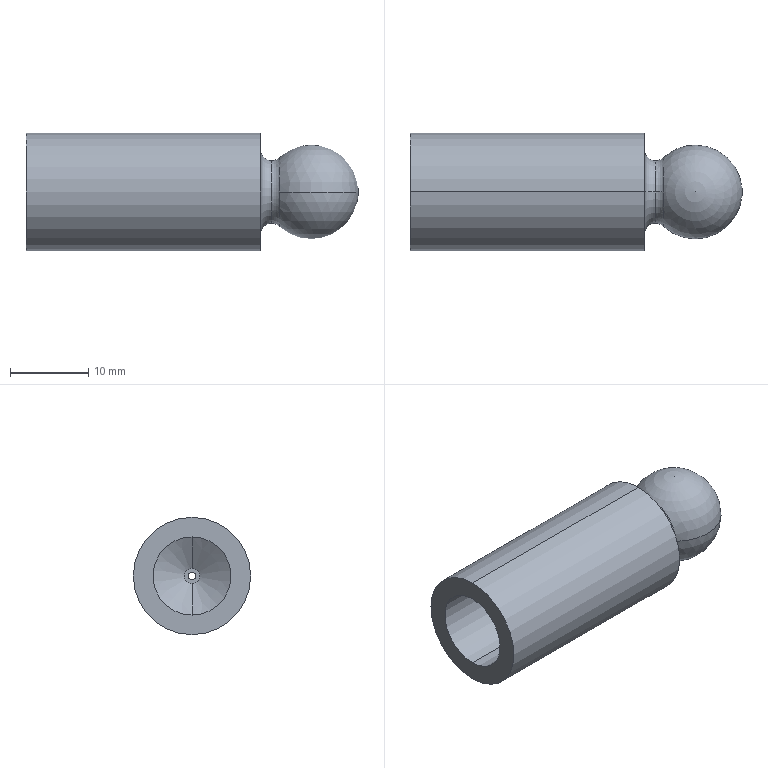Part | SolidWorks | features RevCut 1, Revolution 1 | 1 solid | 19 faces | box 42.479 x 15 x 15 mm | volume 4208 mm3 | cylinder 8 | torus 4 | plane 3 | cone 2 | sphere 2 | commonest cylinder face diameters 1 x2 2 x2 10 x2 15 x2
STEP:
#1=CARTESIAN_POINT('',(30.,0.,5.431));
#2=VERTEX_POINT('',#1);
#3=CARTESIAN_POINT('',(31.43,0.,4.001));
#4=VERTEX_POINT('',#3);
#5=CARTESIAN_POINT('',(31.43,0.,5.431));
#6=DIRECTION('',(0.,-1.,0.));
#7=DIRECTION('',(1.,0.,0.));
#8=AXIS2_PLACEMENT_3D('',#5,#6,#7);
#9=CIRCLE('',#8,1.43);
#10=EDGE_CURVE('',#2,#4,#9,.T.);
#11=ORIENTED_EDGE('',*,*,#10,.T.);
#12=CARTESIAN_POINT('',(31.43,0.,-4.001));
#13=VERTEX_POINT('',#12);
#14=CARTESIAN_POINT('',(31.43,0.,0.));
#15=DIRECTION('',(-1.,0.,0.));
#16=DIRECTION('',(0.,0.,1.));
#17=AXIS2_PLACEMENT_3D('',#14,#15,#16);
#18=CIRCLE('',#17,4.001);
#19=EDGE_CURVE('',#4,#13,#18,.T.);
#20=ORIENTED_EDGE('',*,*,#19,.T.);
#21=CARTESIAN_POINT('',(30.,0.,-5.431));
#22=VERTEX_POINT('',#21);
#23=CARTESIAN_POINT('',(31.43,0.,-5.431));
#24=DIRECTION('',(0.,1.,0.));
#25=DIRECTION('',(0.,0.,1.));
#26=AXIS2_PLACEMENT_3D('',#23,#24,#25);
#27=CIRCLE('',#26,1.43);
#28=EDGE_CURVE('',#22,#13,#27,.T.);
#29=ORIENTED_EDGE('',*,*,#28,.F.);
#30=CARTESIAN_POINT('',(30.,0.,0.));
#31=DIRECTION('',(-1.,0.,0.));
#32=DIRECTION('',(0.,0.,1.));
#33=AXIS2_PLACEMENT_3D('',#30,#31,#32);
#34=CIRCLE('',#33,5.431);
#35=EDGE_CURVE('',#2,#22,#34,.T.);
#36=ORIENTED_EDGE('',*,*,#35,.F.);
#37=EDGE_LOOP('',(#11,#20,#29,#36));
#38=FACE_OUTER_BOUND('',#37,.T.);
#39=CARTESIAN_POINT('',(31.43,0.,0.));
#40=DIRECTION('',(-1.,0.,0.));
#41=DIRECTION('',(0.,0.,1.));
#42=AXIS2_PLACEMENT_3D('',#39,#40,#41);
#43=TOROIDAL_SURFACE('',#42,5.431,1.43);
#44=ADVANCED_FACE('',(#38),#43,.F.);
#45=ORIENTED_EDGE('',*,*,#28,.T.);
#46=CARTESIAN_POINT('',(31.43,0.,0.));
#47=DIRECTION('',(-1.,0.,0.));
#48=DIRECTION('',(0.,0.,1.));
#49=AXIS2_PLACEMENT_3D('',#46,#47,#48);
#50=CIRCLE('',#49,4.001);
#51=EDGE_CURVE('',#13,#4,#50,.T.);
#52=ORIENTED_EDGE('',*,*,#51,.T.);
#53=ORIENTED_EDGE('',*,*,#10,.F.);
#54=CARTESIAN_POINT('',(30.,0.,0.));
#55=DIRECTION('',(-1.,0.,0.));
#56=DIRECTION('',(0.,0.,1.));
#57=AXIS2_PLACEMENT_3D('',#54,#55,#56);
#58=CIRCLE('',#57,5.431);
#59=EDGE_CURVE('',#22,#2,#58,.T.);
#60=ORIENTED_EDGE('',*,*,#59,.F.);
#61=EDGE_LOOP('',(#45,#52,#53,#60));
#62=FACE_OUTER_BOUND('',#61,.T.);
#63=CARTESIAN_POINT('',(31.43,0.,0.));
#64=DIRECTION('',(-1.,0.,0.));
#65=DIRECTION('',(0.,0.,1.));
#66=AXIS2_PLACEMENT_3D('',#63,#64,#65);
#67=TOROIDAL_SURFACE('',#66,5.431,1.43);
#68=ADVANCED_FACE('',(#62),#67,.F.);
#69=CARTESIAN_POINT('',(37.,0.,-1.));
#70=VERTEX_POINT('',#69);
#71=CARTESIAN_POINT('',(37.,0.,1.));
#72=VERTEX_POINT('',#71);
#73=CARTESIAN_POINT('',(37.,0.,0.));
#74=DIRECTION('',(-1.,0.,0.));
#75=DIRECTION('',(0.,0.,1.));
#76=AXIS2_PLACEMENT_3D('',#73,#74,#75);
#77=CIRCLE('',#76,1.);
#78=EDGE_CURVE('',#70,#72,#77,.T.);
#79=ORIENTED_EDGE('',*,*,#78,.F.);
#80=CARTESIAN_POINT('',(27.309,0.,-1.));
#81=VERTEX_POINT('',#80);
#82=CARTESIAN_POINT('',(0.,0.,-1.));
#83=DIRECTION('',(-1.,0.,0.));
#84=VECTOR('',#83,1000.);
#85=LINE('',#82,#84);
#86=EDGE_CURVE('',#70,#81,#85,.T.);
#87=ORIENTED_EDGE('',*,*,#86,.T.);
#88=CARTESIAN_POINT('',(27.309,0.,1.));
#89=VERTEX_POINT('',#88);
#90=CARTESIAN_POINT('',(27.309,0.,0.));
#91=DIRECTION('',(-1.,0.,0.));
#92=DIRECTION('',(0.,0.,1.));
#93=AXIS2_PLACEMENT_3D('',#90,#91,#92);
#94=CIRCLE('',#93,1.);
#95=EDGE_CURVE('',#81,#89,#94,.T.);
#96=ORIENTED_EDGE('',*,*,#95,.T.);
#97=CARTESIAN_POINT('',(0.,0.,1.));
#98=DIRECTION('',(-1.,0.,0.));
#99=VECTOR('',#98,1000.);
#100=LINE('',#97,#99);
#101=EDGE_CURVE('',#72,#89,#100,.T.);
#102=ORIENTED_EDGE('',*,*,#101,.F.);
#103=EDGE_LOOP('',(#79,#87,#96,#102));
#104=FACE_OUTER_BOUND('',#103,.T.);
#105=CARTESIAN_POINT('',(0.,0.,0.));
#106=DIRECTION('',(-1.,0.,0.));
#107=DIRECTION('',(0.,0.,1.));
#108=AXIS2_PLACEMENT_3D('',#105,#106,#107);
#109=CYLINDRICAL_SURFACE('',#108,1.);
#110=ADVANCED_FACE('',(#104),#109,.F.);
#111=ORIENTED_EDGE('',*,*,#95,.F.);
#112=CARTESIAN_POINT('',(25.,0.,-5.));
#113=VERTEX_POINT('',#112);
#114=CARTESIAN_POINT('',(27.309,0.,-1.));
#115=DIRECTION('',(-0.5,0.,-0.866));
#116=VECTOR('',#115,1000.);
#117=LINE('',#114,#116);
#118=EDGE_CURVE('',#81,#113,#117,.T.);
#119=ORIENTED_EDGE('',*,*,#118,.T.);
#120=CARTESIAN_POINT('',(25.,0.,5.));
#121=VERTEX_POINT('',#120);
#122=CARTESIAN_POINT('',(25.,0.,0.));
#123=DIRECTION('',(-1.,0.,0.));
#124=DIRECTION('',(0.,0.,1.));
#125=AXIS2_PLACEMENT_3D('',#122,#123,#124);
#126=CIRCLE('',#125,5.);
#127=EDGE_CURVE('',#113,#121,#126,.T.);
#128=ORIENTED_EDGE('',*,*,#127,.T.);
#129=CARTESIAN_POINT('',(27.309,0.,1.));
#130=DIRECTION('',(-0.5,0.,0.866));
#131=VECTOR('',#130,1000.);
#132=LINE('',#129,#131);
#133=EDGE_CURVE('',#89,#121,#132,.T.);
#134=ORIENTED_EDGE('',*,*,#133,.F.);
#135=EDGE_LOOP('',(#111,#119,#128,#134));
#136=FACE_OUTER_BOUND('',#135,.T.);
#137=CARTESIAN_POINT('',(27.309,0.,0.));
#138=DIRECTION('',(-1.,0.,0.));
#139=DIRECTION('',(0.,0.,1.));
#140=AXIS2_PLACEMENT_3D('',#137,#138,#139);
#141=CONICAL_SURFACE('',#140,1.,1.047);
#142=ADVANCED_FACE('',(#136),#141,.F.);
#143=ORIENTED_EDGE('',*,*,#127,.F.);
#144=CARTESIAN_POINT('',(0.,0.,-5.));
#145=VERTEX_POINT('',#144);
#146=CARTESIAN_POINT('',(0.,0.,-5.));
#147=DIRECTION('',(-1.,0.,0.));
#148=VECTOR('',#147,1000.);
#149=LINE('',#146,#148);
#150=EDGE_CURVE('',#113,#145,#149,.T.);
#151=ORIENTED_EDGE('',*,*,#150,.T.);
#152=CARTESIAN_POINT('',(0.,0.,5.));
#153=VERTEX_POINT('',#152);
#154=CARTESIAN_POINT('',(0.,0.,0.));
#155=DIRECTION('',(-1.,0.,0.));
#156=DIRECTION('',(0.,0.,1.));
#157=AXIS2_PLACEMENT_3D('',#154,#155,#156);
#158=CIRCLE('',#157,5.);
#159=EDGE_CURVE('',#145,#153,#158,.T.);
#160=ORIENTED_EDGE('',*,*,#159,.T.);
#161=CARTESIAN_POINT('',(0.,0.,5.));
#162=DIRECTION('',(-1.,0.,0.));
#163=VECTOR('',#162,1000.);
#164=LINE('',#161,#163);
#165=EDGE_CURVE('',#121,#153,#164,.T.);
#166=ORIENTED_EDGE('',*,*,#165,.F.);
#167=EDGE_LOOP('',(#143,#151,#160,#166));
#168=FACE_OUTER_BOUND('',#167,.T.);
#169=CARTESIAN_POINT('',(0.,0.,0.));
#170=DIRECTION('',(-1.,0.,0.));
#171=DIRECTION('',(0.,0.,1.));
#172=AXIS2_PLACEMENT_3D('',#169,#170,#171);
#173=CYLINDRICAL_SURFACE('',#172,5.);
#174=ADVANCED_FACE('',(#168),#173,.F.);
#175=CARTESIAN_POINT('',(42.479,-0.5,0.));
#176=VERTEX_POINT('',#175);
#177=CARTESIAN_POINT('',(42.479,0.,-0.5));
#178=VERTEX_POINT('',#177);
#179=CARTESIAN_POINT('',(42.479,0.,0.));
#180=DIRECTION('',(1.,0.,0.));
#181=DIRECTION('',(0.,0.,1.));
#182=AXIS2_PLACEMENT_3D('',#179,#180,#181);
#183=CIRCLE('',#182,0.5);
#184=EDGE_CURVE('',#176,#178,#183,.T.);
#185=ORIENTED_EDGE('',*,*,#184,.T.);
#186=CARTESIAN_POINT('',(37.,0.,-0.5));
#187=VERTEX_POINT('',#186);
#188=CARTESIAN_POINT('',(0.,0.,-0.5));
#189=DIRECTION('',(-1.,0.,0.));
#190=VECTOR('',#189,1000.);
#191=LINE('',#188,#190);
#192=EDGE_CURVE('',#178,#187,#191,.T.);
#193=ORIENTED_EDGE('',*,*,#192,.T.);
#194=CARTESIAN_POINT('',(37.,0.,0.5));
#195=VERTEX_POINT('',#194);
#196=CARTESIAN_POINT('',(37.,0.,0.));
#197=DIRECTION('',(-1.,0.,0.));
#198=DIRECTION('',(0.,0.,1.));
#199=AXIS2_PLACEMENT_3D('',#196,#197,#198);
#200=CIRCLE('',#199,0.5);
#201=EDGE_CURVE('',#187,#195,#200,.T.);
#202=ORIENTED_EDGE('',*,*,#201,.T.);
#203=CARTESIAN_POINT('',(42.479,0.,0.5));
#204=VERTEX_POINT('',#203);
#205=CARTESIAN_POINT('',(0.,0.,0.5));
#206=DIRECTION('',(-1.,0.,0.));
#207=VECTOR('',#206,1000.);
#208=LINE('',#205,#207);
#209=EDGE_CURVE('',#204,#195,#208,.T.);
#210=ORIENTED_EDGE('',*,*,#209,.F.);
#211=CARTESIAN_POINT('',(42.479,0.,0.));
#212=DIRECTION('',(1.,0.,0.));
#213=DIRECTION('',(0.,0.,1.));
#214=AXIS2_PLACEMENT_3D('',#211,#212,#213);
#215=CIRCLE('',#214,0.5);
#216=EDGE_CURVE('',#204,#176,#215,.T.);
#217=ORIENTED_EDGE('',*,*,#216,.T.);
#218=EDGE_LOOP('',(#185,#193,#202,#210,#217));
#219=FACE_OUTER_BOUND('',#218,.T.);
#220=CARTESIAN_POINT('',(0.,0.,0.));
#221=DIRECTION('',(-1.,0.,0.));
#222=DIRECTION('',(0.,0.,1.));
#223=AXIS2_PLACEMENT_3D('',#220,#221,#222);
#224=CYLINDRICAL_SURFACE('',#223,0.5);
#225=ADVANCED_FACE('',(#219),#224,.F.);
#226=ORIENTED_EDGE('',*,*,#51,.F.);
#227=CARTESIAN_POINT('',(32.406,0.,-4.386));
#228=VERTEX_POINT('',#227);
#229=CARTESIAN_POINT('',(31.43,0.,-5.431));
#230=DIRECTION('',(0.,1.,0.));
#231=DIRECTION('',(0.,0.,1.));
#232=AXIS2_PLACEMENT_3D('',#229,#230,#231);
#233=CIRCLE('',#232,1.43);
#234=EDGE_CURVE('',#13,#228,#233,.T.);
#235=ORIENTED_EDGE('',*,*,#234,.T.);
#236=CARTESIAN_POINT('',(32.406,-4.386,0.));
#237=VERTEX_POINT('',#236);
#238=CARTESIAN_POINT('',(32.406,0.,0.));
#239=DIRECTION('',(-1.,0.,0.));
#240=DIRECTION('',(0.,0.,1.));
#241=AXIS2_PLACEMENT_3D('',#238,#239,#240);
#242=CIRCLE('',#241,4.386);
#243=EDGE_CURVE('',#228,#237,#242,.T.);
#244=ORIENTED_EDGE('',*,*,#243,.T.);
#245=CARTESIAN_POINT('',(32.406,0.,4.386));
#246=VERTEX_POINT('',#245);
#247=CARTESIAN_POINT('',(32.406,0.,0.));
#248=DIRECTION('',(-1.,0.,0.));
#249=DIRECTION('',(0.,0.,1.));
#250=AXIS2_PLACEMENT_3D('',#247,#248,#249);
#251=CIRCLE('',#250,4.386);
#252=EDGE_CURVE('',#237,#246,#251,.T.);
#253=ORIENTED_EDGE('',*,*,#252,.T.);
#254=CARTESIAN_POINT('',(31.43,0.,5.431));
#255=DIRECTION('',(0.,-1.,0.));
#256=DIRECTION('',(1.,0.,0.));
#257=AXIS2_PLACEMENT_3D('',#254,#255,#256);
#258=CIRCLE('',#257,1.43);
#259=EDGE_CURVE('',#4,#246,#258,.T.);
#260=ORIENTED_EDGE('',*,*,#259,.F.);
#261=EDGE_LOOP('',(#226,#235,#244,#253,#260));
#262=FACE_OUTER_BOUND('',#261,.T.);
#263=CARTESIAN_POINT('',(31.43,0.,0.));
#264=DIRECTION('',(-1.,0.,0.));
#265=DIRECTION('',(0.,0.,1.));
#266=AXIS2_PLACEMENT_3D('',#263,#264,#265);
#267=TOROIDAL_SURFACE('',#266,5.431,1.43);
#268=ADVANCED_FACE('',(#262),#267,.F.);
#269=CARTESIAN_POINT('',(30.,0.,7.5));
#270=VERTEX_POINT('',#269);
#271=CARTESIAN_POINT('',(30.,0.,-7.5));
#272=VERTEX_POINT('',#271);
#273=CARTESIAN_POINT('',(30.,0.,0.));
#274=DIRECTION('',(-1.,0.,0.));
#275=DIRECTION('',(0.,0.,1.));
#276=AXIS2_PLACEMENT_3D('',#273,#274,#275);
#277=CIRCLE('',#276,7.5);
#278=EDGE_CURVE('',#270,#272,#277,.T.);
#279=ORIENTED_EDGE('',*,*,#278,.T.);
#280=CARTESIAN_POINT('',(0.,0.,-7.5));
#281=VERTEX_POINT('',#280);
#282=CARTESIAN_POINT('',(0.,0.,-7.5));
#283=DIRECTION('',(-1.,0.,0.));
#284=VECTOR('',#283,1000.);
#285=LINE('',#282,#284);
#286=EDGE_CURVE('',#272,#281,#285,.T.);
#287=ORIENTED_EDGE('',*,*,#286,.T.);
#288=CARTESIAN_POINT('',(0.,0.,7.5));
#289=VERTEX_POINT('',#288);
#290=CARTESIAN_POINT('',(0.,0.,0.));
#291=DIRECTION('',(-1.,0.,0.));
#292=DIRECTION('',(0.,0.,1.));
#293=AXIS2_PLACEMENT_3D('',#290,#291,#292);
#294=CIRCLE('',#293,7.5);
#295=EDGE_CURVE('',#289,#281,#294,.T.);
#296=ORIENTED_EDGE('',*,*,#295,.F.);
#297=CARTESIAN_POINT('',(0.,0.,7.5));
#298=DIRECTION('',(-1.,0.,0.));
#299=VECTOR('',#298,1000.);
#300=LINE('',#297,#299);
#301=EDGE_CURVE('',#270,#289,#300,.T.);
#302=ORIENTED_EDGE('',*,*,#301,.F.);
#303=EDGE_LOOP('',(#279,#287,#296,#302));
#304=FACE_OUTER_BOUND('',#303,.T.);
#305=CARTESIAN_POINT('',(0.,0.,0.));
#306=DIRECTION('',(-1.,0.,0.));
#307=DIRECTION('',(0.,0.,1.));
#308=AXIS2_PLACEMENT_3D('',#305,#306,#307);
#309=CYLINDRICAL_SURFACE('',#308,7.5);
#310=ADVANCED_FACE('',(#304),#309,.T.);
#311=ORIENTED_EDGE('',*,*,#184,.F.);
#312=CARTESIAN_POINT('',(36.5,0.,0.));
#313=DIRECTION('',(0.,0.,-1.));
#314=DIRECTION('',(0.,1.,0.));
#315=AXIS2_PLACEMENT_3D('',#312,#313,#314);
#316=CIRCLE('',#315,6.);
#317=EDGE_CURVE('',#176,#237,#316,.T.);
#318=ORIENTED_EDGE('',*,*,#317,.T.);
#319=ORIENTED_EDGE('',*,*,#243,.F.);
#320=CARTESIAN_POINT('',(32.406,4.386,0.));
#321=VERTEX_POINT('',#320);
#322=CARTESIAN_POINT('',(32.406,0.,0.));
#323=DIRECTION('',(-1.,0.,0.));
#324=DIRECTION('',(0.,0.,1.));
#325=AXIS2_PLACEMENT_3D('',#322,#323,#324);
#326=CIRCLE('',#325,4.386);
#327=EDGE_CURVE('',#321,#228,#326,.T.);
#328=ORIENTED_EDGE('',*,*,#327,.F.);
#329=CARTESIAN_POINT('',(42.479,0.5,0.));
#330=VERTEX_POINT('',#329);
#331=CARTESIAN_POINT('',(36.5,0.,0.));
#332=DIRECTION('',(0.,0.,1.));
#333=DIRECTION('',(1.,0.,0.));
#334=AXIS2_PLACEMENT_3D('',#331,#332,#333);
#335=CIRCLE('',#334,6.);
#336=EDGE_CURVE('',#330,#321,#335,.T.);
#337=ORIENTED_EDGE('',*,*,#336,.F.);
#338=CARTESIAN_POINT('',(42.479,0.,0.));
#339=DIRECTION('',(1.,0.,0.));
#340=DIRECTION('',(0.,0.,1.));
#341=AXIS2_PLACEMENT_3D('',#338,#339,#340);
#342=CIRCLE('',#341,0.5);
#343=EDGE_CURVE('',#178,#330,#342,.T.);
#344=ORIENTED_EDGE('',*,*,#343,.F.);
#345=EDGE_LOOP('',(#311,#318,#319,#328,#337,#344));
#346=FACE_OUTER_BOUND('',#345,.T.);
#347=CARTESIAN_POINT('',(36.5,0.,0.));
#348=DIRECTION('',(0.,0.,-1.));
#349=DIRECTION('',(0.,1.,0.));
#350=AXIS2_PLACEMENT_3D('',#347,#348,#349);
#351=SPHERICAL_SURFACE('',#350,6.);
#352=ADVANCED_FACE('',(#346),#351,.T.);
#353=ORIENTED_EDGE('',*,*,#317,.F.);
#354=ORIENTED_EDGE('',*,*,#216,.F.);
#355=CARTESIAN_POINT('',(42.479,0.,0.));
#356=DIRECTION('',(1.,0.,0.));
#357=DIRECTION('',(0.,0.,1.));
#358=AXIS2_PLACEMENT_3D('',#355,#356,#357);
#359=CIRCLE('',#358,0.5);
#360=EDGE_CURVE('',#330,#204,#359,.T.);
#361=ORIENTED_EDGE('',*,*,#360,.F.);
#362=ORIENTED_EDGE('',*,*,#336,.T.);
#363=CARTESIAN_POINT('',(32.406,0.,0.));
#364=DIRECTION('',(-1.,0.,0.));
#365=DIRECTION('',(0.,0.,1.));
#366=AXIS2_PLACEMENT_3D('',#363,#364,#365);
#367=CIRCLE('',#366,4.386);
#368=EDGE_CURVE('',#246,#321,#367,.T.);
#369=ORIENTED_EDGE('',*,*,#368,.F.);
#370=ORIENTED_EDGE('',*,*,#252,.F.);
#371=EDGE_LOOP('',(#353,#354,#361,#362,#369,#370));
#372=FACE_OUTER_BOUND('',#371,.T.);
#373=CARTESIAN_POINT('',(36.5,0.,0.));
#374=DIRECTION('',(0.,0.,-1.));
#375=DIRECTION('',(0.,1.,0.));
#376=AXIS2_PLACEMENT_3D('',#373,#374,#375);
#377=SPHERICAL_SURFACE('',#376,6.);
#378=ADVANCED_FACE('',(#372),#377,.T.);
#379=CARTESIAN_POINT('',(0.,0.,0.));
#380=DIRECTION('',(-1.,0.,0.));
#381=DIRECTION('',(0.,0.,1.));
#382=AXIS2_PLACEMENT_3D('',#379,#380,#381);
#383=CIRCLE('',#382,5.);
#384=EDGE_CURVE('',#153,#145,#383,.T.);
#385=ORIENTED_EDGE('',*,*,#384,.F.);
#386=ORIENTED_EDGE('',*,*,#159,.F.);
#387=EDGE_LOOP('',(#385,#386));
#388=FACE_BOUND('',#387,.T.);
#389=ORIENTED_EDGE('',*,*,#295,.T.);
#390=CARTESIAN_POINT('',(0.,0.,0.));
#391=DIRECTION('',(-1.,0.,0.));
#392=DIRECTION('',(0.,0.,1.));
#393=AXIS2_PLACEMENT_3D('',#390,#391,#392);
#394=CIRCLE('',#393,7.5);
#395=EDGE_CURVE('',#281,#289,#394,.T.);
#396=ORIENTED_EDGE('',*,*,#395,.T.);
#397=EDGE_LOOP('',(#389,#396));
#398=FACE_OUTER_BOUND('',#397,.T.);
#399=CARTESIAN_POINT('',(0.,0.,0.));
#400=DIRECTION('',(1.,0.,0.));
#401=DIRECTION('',(0.,0.,-1.));
#402=AXIS2_PLACEMENT_3D('',#399,#400,#401);
#403=PLANE('',#402);
#404=ADVANCED_FACE('',(#388,#398),#403,.F.);
#405=ORIENTED_EDGE('',*,*,#286,.F.);
#406=CARTESIAN_POINT('',(30.,0.,0.));
#407=DIRECTION('',(-1.,0.,0.));
#408=DIRECTION('',(0.,0.,1.));
#409=AXIS2_PLACEMENT_3D('',#406,#407,#408);
#410=CIRCLE('',#409,7.5);
#411=EDGE_CURVE('',#272,#270,#410,.T.);
#412=ORIENTED_EDGE('',*,*,#411,.T.);
#413=ORIENTED_EDGE('',*,*,#301,.T.);
#414=ORIENTED_EDGE('',*,*,#395,.F.);
#415=EDGE_LOOP('',(#405,#412,#413,#414));
#416=FACE_OUTER_BOUND('',#415,.T.);
#417=CARTESIAN_POINT('',(0.,0.,0.));
#418=DIRECTION('',(-1.,0.,0.));
#419=DIRECTION('',(0.,0.,1.));
#420=AXIS2_PLACEMENT_3D('',#417,#418,#419);
#421=CYLINDRICAL_SURFACE('',#420,7.5);
#422=ADVANCED_FACE('',(#416),#421,.T.);
#423=ORIENTED_EDGE('',*,*,#278,.F.);
#424=ORIENTED_EDGE('',*,*,#411,.F.);
#425=EDGE_LOOP('',(#423,#424));
#426=FACE_OUTER_BOUND('',#425,.T.);
#427=ORIENTED_EDGE('',*,*,#35,.T.);
#428=ORIENTED_EDGE('',*,*,#59,.T.);
#429=EDGE_LOOP('',(#427,#428));
#430=FACE_BOUND('',#429,.T.);
#431=CARTESIAN_POINT('',(30.,7.5,0.));
#432=DIRECTION('',(-1.,0.,0.));
#433=DIRECTION('',(0.,0.,1.));
#434=AXIS2_PLACEMENT_3D('',#431,#432,#433);
#435=PLANE('',#434);
#436=ADVANCED_FACE('',(#426,#430),#435,.F.);
#437=ORIENTED_EDGE('',*,*,#19,.F.);
#438=ORIENTED_EDGE('',*,*,#259,.T.);
#439=ORIENTED_EDGE('',*,*,#368,.T.);
#440=ORIENTED_EDGE('',*,*,#327,.T.);
#441=ORIENTED_EDGE('',*,*,#234,.F.);
#442=EDGE_LOOP('',(#437,#438,#439,#440,#441));
#443=FACE_OUTER_BOUND('',#442,.T.);
#444=CARTESIAN_POINT('',(31.43,0.,0.));
#445=DIRECTION('',(-1.,0.,0.));
#446=DIRECTION('',(0.,0.,1.));
#447=AXIS2_PLACEMENT_3D('',#444,#445,#446);
#448=TOROIDAL_SURFACE('',#447,5.431,1.43);
#449=ADVANCED_FACE('',(#443),#448,.F.);
#450=ORIENTED_EDGE('',*,*,#192,.F.);
#451=ORIENTED_EDGE('',*,*,#343,.T.);
#452=ORIENTED_EDGE('',*,*,#360,.T.);
#453=ORIENTED_EDGE('',*,*,#209,.T.);
#454=CARTESIAN_POINT('',(37.,0.,0.));
#455=DIRECTION('',(-1.,0.,0.));
#456=DIRECTION('',(0.,0.,1.));
#457=AXIS2_PLACEMENT_3D('',#454,#455,#456);
#458=CIRCLE('',#457,0.5);
#459=EDGE_CURVE('',#195,#187,#458,.T.);
#460=ORIENTED_EDGE('',*,*,#459,.T.);
#461=EDGE_LOOP('',(#450,#451,#452,#453,#460));
#462=FACE_OUTER_BOUND('',#461,.T.);
#463=CARTESIAN_POINT('',(0.,0.,0.));
#464=DIRECTION('',(-1.,0.,0.));
#465=DIRECTION('',(0.,0.,1.));
#466=AXIS2_PLACEMENT_3D('',#463,#464,#465);
#467=CYLINDRICAL_SURFACE('',#466,0.5);
#468=ADVANCED_FACE('',(#462),#467,.F.);
#469=ORIENTED_EDGE('',*,*,#150,.F.);
#470=CARTESIAN_POINT('',(25.,0.,0.));
#471=DIRECTION('',(-1.,0.,0.));
#472=DIRECTION('',(0.,0.,1.));
#473=AXIS2_PLACEMENT_3D('',#470,#471,#472);
#474=CIRCLE('',#473,5.);
#475=EDGE_CURVE('',#121,#113,#474,.T.);
#476=ORIENTED_EDGE('',*,*,#475,.F.);
#477=ORIENTED_EDGE('',*,*,#165,.T.);
#478=ORIENTED_EDGE('',*,*,#384,.T.);
#479=EDGE_LOOP('',(#469,#476,#477,#478));
#480=FACE_OUTER_BOUND('',#479,.T.);
#481=CARTESIAN_POINT('',(0.,0.,0.));
#482=DIRECTION('',(-1.,0.,0.));
#483=DIRECTION('',(0.,0.,1.));
#484=AXIS2_PLACEMENT_3D('',#481,#482,#483);
#485=CYLINDRICAL_SURFACE('',#484,5.);
#486=ADVANCED_FACE('',(#480),#485,.F.);
#487=ORIENTED_EDGE('',*,*,#118,.F.);
#488=CARTESIAN_POINT('',(27.309,0.,0.));
#489=DIRECTION('',(-1.,0.,0.));
#490=DIRECTION('',(0.,0.,1.));
#491=AXIS2_PLACEMENT_3D('',#488,#489,#490);
#492=CIRCLE('',#491,1.);
#493=EDGE_CURVE('',#89,#81,#492,.T.);
#494=ORIENTED_EDGE('',*,*,#493,.F.);
#495=ORIENTED_EDGE('',*,*,#133,.T.);
#496=ORIENTED_EDGE('',*,*,#475,.T.);
#497=EDGE_LOOP('',(#487,#494,#495,#496));
#498=FACE_OUTER_BOUND('',#497,.T.);
#499=CARTESIAN_POINT('',(27.309,0.,0.));
#500=DIRECTION('',(-1.,0.,0.));
#501=DIRECTION('',(0.,0.,1.));
#502=AXIS2_PLACEMENT_3D('',#499,#500,#501);
#503=CONICAL_SURFACE('',#502,1.,1.047);
#504=ADVANCED_FACE('',(#498),#503,.F.);
#505=ORIENTED_EDGE('',*,*,#86,.F.);
#506=CARTESIAN_POINT('',(37.,0.,0.));
#507=DIRECTION('',(-1.,0.,0.));
#508=DIRECTION('',(0.,0.,1.));
#509=AXIS2_PLACEMENT_3D('',#506,#507,#508);
#510=CIRCLE('',#509,1.);
#511=EDGE_CURVE('',#72,#70,#510,.T.);
#512=ORIENTED_EDGE('',*,*,#511,.F.);
#513=ORIENTED_EDGE('',*,*,#101,.T.);
#514=ORIENTED_EDGE('',*,*,#493,.T.);
#515=EDGE_LOOP('',(#505,#512,#513,#514));
#516=FACE_OUTER_BOUND('',#515,.T.);
#517=CARTESIAN_POINT('',(0.,0.,0.));
#518=DIRECTION('',(-1.,0.,0.));
#519=DIRECTION('',(0.,0.,1.));
#520=AXIS2_PLACEMENT_3D('',#517,#518,#519);
#521=CYLINDRICAL_SURFACE('',#520,1.);
#522=ADVANCED_FACE('',(#516),#521,.F.);
#523=ORIENTED_EDGE('',*,*,#511,.T.);
#524=ORIENTED_EDGE('',*,*,#78,.T.);
#525=EDGE_LOOP('',(#523,#524));
#526=FACE_OUTER_BOUND('',#525,.T.);
#527=ORIENTED_EDGE('',*,*,#459,.F.);
#528=ORIENTED_EDGE('',*,*,#201,.F.);
#529=EDGE_LOOP('',(#527,#528));
#530=FACE_BOUND('',#529,.T.);
#531=CARTESIAN_POINT('',(37.,0.5,0.));
#532=DIRECTION('',(-1.,0.,0.));
#533=DIRECTION('',(0.,0.,1.));
#534=AXIS2_PLACEMENT_3D('',#531,#532,#533);
#535=PLANE('',#534);
#536=ADVANCED_FACE('',(#526,#530),#535,.T.);
#537=CLOSED_SHELL('',(#44,#68,#110,#142,#174,#225,#268,#310,#352,#378,#404,#422,#436,#449,#468,#486,#504,#522,#536));
#538=MANIFOLD_SOLID_BREP('',#537);
#539=CARTESIAN_POINT('',(0.,0.,0.));
#540=DIRECTION('',(0.,0.,1.));
#541=DIRECTION('',(1.,0.,0.));
#542=AXIS2_PLACEMENT_3D('',#539,#540,#541);
#543=(LENGTH_UNIT()NAMED_UNIT(*)SI_UNIT(.MILLI.,.METRE.));
#544=UNCERTAINTY_MEASURE_WITH_UNIT(LENGTH_MEASURE(0.00001),#543,'','');
#545=(NAMED_UNIT(*)PLANE_ANGLE_UNIT()SI_UNIT($,.RADIAN.));
#546=(NAMED_UNIT(*)SI_UNIT($,.STERADIAN.)SOLID_ANGLE_UNIT());
#547=(GEOMETRIC_REPRESENTATION_CONTEXT(3)GLOBAL_UNCERTAINTY_ASSIGNED_CONTEXT((#544))GLOBAL_UNIT_ASSIGNED_CONTEXT((#543,#545,#546))REPRESENTATION_CONTEXT('',''));
#548=ADVANCED_BREP_SHAPE_REPRESENTATION('',(#538,#542),#547);